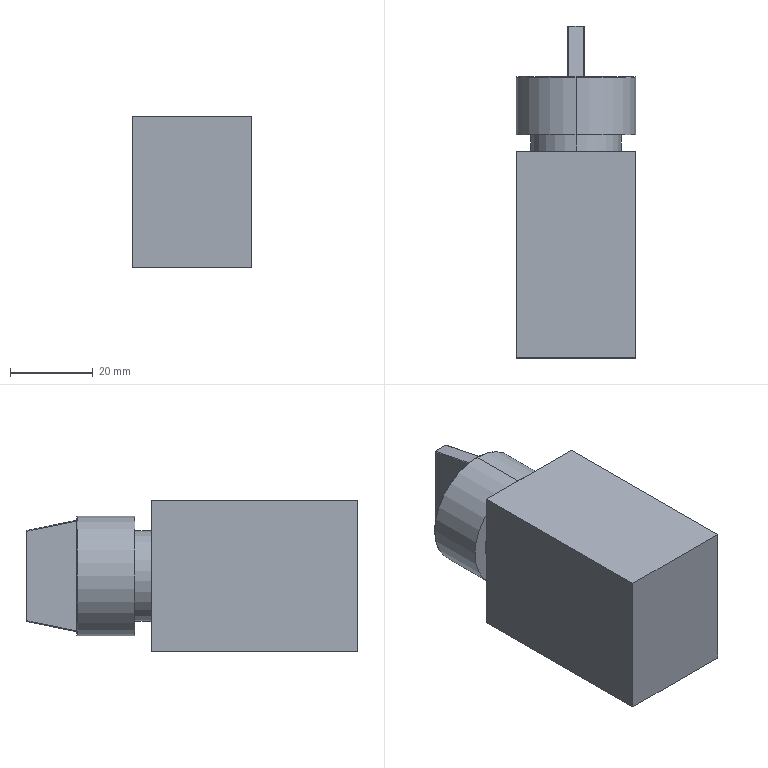Part | SolidWorks | features ICE 4, Extrusion 1, Fillet 1 | 1 solid | 25 faces | box 29 x 80.3 x 36.6 mm | volume 65042 mm3 | plane 13 | cylinder 10 | torus 2 | commonest cylinder face diameters 0.4 x6 22 x2 29 x2
STEP:
#1=CARTESIAN_POINT('',(0.,13.8,-14.5));
#2=VERTEX_POINT('',#1);
#3=CARTESIAN_POINT('',(0.,13.8,14.5));
#4=VERTEX_POINT('',#3);
#5=CARTESIAN_POINT('',(0.,13.8,0.));
#6=DIRECTION('',(0.,-1.,0.));
#7=DIRECTION('',(0.,0.,1.));
#8=AXIS2_PLACEMENT_3D('',#5,#6,#7);
#9=CIRCLE('',#8,14.5);
#10=EDGE_CURVE('',#2,#4,#9,.T.);
#11=ORIENTED_EDGE('',*,*,#10,.F.);
#12=CARTESIAN_POINT('',(0.,14.,-14.3));
#13=VERTEX_POINT('',#12);
#14=CARTESIAN_POINT('',(0.,13.8,-14.3));
#15=DIRECTION('',(1.,0.,0.));
#16=DIRECTION('',(0.,0.,-1.));
#17=AXIS2_PLACEMENT_3D('',#14,#15,#16);
#18=CIRCLE('',#17,0.2);
#19=EDGE_CURVE('',#2,#13,#18,.T.);
#20=ORIENTED_EDGE('',*,*,#19,.T.);
#21=CARTESIAN_POINT('',(0.,14.,14.3));
#22=VERTEX_POINT('',#21);
#23=CARTESIAN_POINT('',(0.,14.,0.));
#24=DIRECTION('',(0.,1.,0.));
#25=DIRECTION('',(0.,0.,1.));
#26=AXIS2_PLACEMENT_3D('',#23,#24,#25);
#27=CIRCLE('',#26,14.3);
#28=EDGE_CURVE('',#22,#13,#27,.T.);
#29=ORIENTED_EDGE('',*,*,#28,.F.);
#30=CARTESIAN_POINT('',(0.,13.8,14.3));
#31=DIRECTION('',(-1.,0.,0.));
#32=DIRECTION('',(0.,0.,1.));
#33=AXIS2_PLACEMENT_3D('',#30,#31,#32);
#34=CIRCLE('',#33,0.2);
#35=EDGE_CURVE('',#4,#22,#34,.T.);
#36=ORIENTED_EDGE('',*,*,#35,.F.);
#37=EDGE_LOOP('',(#11,#20,#29,#36));
#38=FACE_OUTER_BOUND('',#37,.T.);
#39=CARTESIAN_POINT('',(0.,13.8,0.));
#40=DIRECTION('',(0.,1.,0.));
#41=DIRECTION('',(0.,0.,1.));
#42=AXIS2_PLACEMENT_3D('',#39,#40,#41);
#43=TOROIDAL_SURFACE('',#42,14.3,0.2);
#44=ADVANCED_FACE('',(#38),#43,.T.);
#45=CARTESIAN_POINT('',(0.,-4.,-11.));
#46=VERTEX_POINT('',#45);
#47=CARTESIAN_POINT('',(0.,-4.,11.));
#48=VERTEX_POINT('',#47);
#49=CARTESIAN_POINT('',(0.,-4.,0.));
#50=DIRECTION('',(0.,-1.,0.));
#51=DIRECTION('',(0.,0.,-1.));
#52=AXIS2_PLACEMENT_3D('',#49,#50,#51);
#53=CIRCLE('',#52,11.);
#54=EDGE_CURVE('',#46,#48,#53,.T.);
#55=ORIENTED_EDGE('',*,*,#54,.F.);
#56=CARTESIAN_POINT('',(0.,0.,-11.));
#57=VERTEX_POINT('',#56);
#58=CARTESIAN_POINT('',(0.,-4.,-11.));
#59=DIRECTION('',(0.,1.,0.));
#60=VECTOR('',#59,1000.);
#61=LINE('',#58,#60);
#62=EDGE_CURVE('',#46,#57,#61,.T.);
#63=ORIENTED_EDGE('',*,*,#62,.T.);
#64=CARTESIAN_POINT('',(0.,0.,11.));
#65=VERTEX_POINT('',#64);
#66=CARTESIAN_POINT('',(0.,0.,0.));
#67=DIRECTION('',(0.,-1.,0.));
#68=DIRECTION('',(0.,0.,1.));
#69=AXIS2_PLACEMENT_3D('',#66,#67,#68);
#70=CIRCLE('',#69,11.);
#71=EDGE_CURVE('',#57,#65,#70,.T.);
#72=ORIENTED_EDGE('',*,*,#71,.T.);
#73=CARTESIAN_POINT('',(0.,-4.,11.));
#74=DIRECTION('',(0.,1.,0.));
#75=VECTOR('',#74,1000.);
#76=LINE('',#73,#75);
#77=EDGE_CURVE('',#48,#65,#76,.T.);
#78=ORIENTED_EDGE('',*,*,#77,.F.);
#79=EDGE_LOOP('',(#55,#63,#72,#78));
#80=FACE_OUTER_BOUND('',#79,.T.);
#81=CARTESIAN_POINT('',(0.,-4.,0.));
#82=DIRECTION('',(0.,1.,0.));
#83=DIRECTION('',(0.,0.,1.));
#84=AXIS2_PLACEMENT_3D('',#81,#82,#83);
#85=CYLINDRICAL_SURFACE('',#84,11.);
#86=ADVANCED_FACE('',(#80),#85,.T.);
#87=ORIENTED_EDGE('',*,*,#10,.T.);
#88=CARTESIAN_POINT('',(0.,0.,14.5));
#89=VERTEX_POINT('',#88);
#90=CARTESIAN_POINT('',(0.,14.,14.5));
#91=DIRECTION('',(0.,-1.,0.));
#92=VECTOR('',#91,1000.);
#93=LINE('',#90,#92);
#94=EDGE_CURVE('',#4,#89,#93,.T.);
#95=ORIENTED_EDGE('',*,*,#94,.T.);
#96=CARTESIAN_POINT('',(0.,0.,-14.5));
#97=VERTEX_POINT('',#96);
#98=CARTESIAN_POINT('',(0.,0.,0.));
#99=DIRECTION('',(0.,1.,0.));
#100=DIRECTION('',(0.,0.,1.));
#101=AXIS2_PLACEMENT_3D('',#98,#99,#100);
#102=CIRCLE('',#101,14.5);
#103=EDGE_CURVE('',#89,#97,#102,.T.);
#104=ORIENTED_EDGE('',*,*,#103,.T.);
#105=CARTESIAN_POINT('',(0.,14.,-14.5));
#106=DIRECTION('',(0.,-1.,0.));
#107=VECTOR('',#106,1000.);
#108=LINE('',#105,#107);
#109=EDGE_CURVE('',#2,#97,#108,.T.);
#110=ORIENTED_EDGE('',*,*,#109,.F.);
#111=EDGE_LOOP('',(#87,#95,#104,#110));
#112=FACE_OUTER_BOUND('',#111,.T.);
#113=CARTESIAN_POINT('',(0.,14.,0.));
#114=DIRECTION('',(0.,-1.,0.));
#115=DIRECTION('',(0.,0.,-1.));
#116=AXIS2_PLACEMENT_3D('',#113,#114,#115);
#117=CYLINDRICAL_SURFACE('',#116,14.5);
#118=ADVANCED_FACE('',(#112),#117,.T.);
#119=CARTESIAN_POINT('',(0.,0.,0.));
#120=DIRECTION('',(0.,1.,0.));
#121=DIRECTION('',(0.,0.,1.));
#122=AXIS2_PLACEMENT_3D('',#119,#120,#121);
#123=CIRCLE('',#122,14.5);
#124=EDGE_CURVE('',#97,#89,#123,.T.);
#125=ORIENTED_EDGE('',*,*,#124,.F.);
#126=ORIENTED_EDGE('',*,*,#103,.F.);
#127=EDGE_LOOP('',(#125,#126));
#128=FACE_OUTER_BOUND('',#127,.T.);
#129=CARTESIAN_POINT('',(0.,0.,0.));
#130=DIRECTION('',(0.,-1.,0.));
#131=DIRECTION('',(0.,0.,1.));
#132=AXIS2_PLACEMENT_3D('',#129,#130,#131);
#133=CIRCLE('',#132,11.);
#134=EDGE_CURVE('',#65,#57,#133,.T.);
#135=ORIENTED_EDGE('',*,*,#134,.F.);
#136=ORIENTED_EDGE('',*,*,#71,.F.);
#137=EDGE_LOOP('',(#135,#136));
#138=FACE_BOUND('',#137,.T.);
#139=CARTESIAN_POINT('',(0.,0.,0.));
#140=DIRECTION('',(0.,1.,0.));
#141=DIRECTION('',(0.,0.,1.));
#142=AXIS2_PLACEMENT_3D('',#139,#140,#141);
#143=PLANE('',#142);
#144=ADVANCED_FACE('',(#128,#138),#143,.F.);
#145=ORIENTED_EDGE('',*,*,#28,.T.);
#146=CARTESIAN_POINT('',(0.,14.,0.));
#147=DIRECTION('',(0.,1.,0.));
#148=DIRECTION('',(0.,0.,1.));
#149=AXIS2_PLACEMENT_3D('',#146,#147,#148);
#150=CIRCLE('',#149,14.3);
#151=EDGE_CURVE('',#13,#22,#150,.T.);
#152=ORIENTED_EDGE('',*,*,#151,.T.);
#153=EDGE_LOOP('',(#145,#152));
#154=FACE_OUTER_BOUND('',#153,.T.);
#155=CARTESIAN_POINT('',(-1.8,14.,13.5));
#156=VERTEX_POINT('',#155);
#157=CARTESIAN_POINT('',(1.8,14.,13.5));
#158=VERTEX_POINT('',#157);
#159=CARTESIAN_POINT('',(-2.,14.,13.5));
#160=DIRECTION('',(1.,0.,0.));
#161=VECTOR('',#160,1000.);
#162=LINE('',#159,#161);
#163=EDGE_CURVE('',#156,#158,#162,.T.);
#164=ORIENTED_EDGE('',*,*,#163,.F.);
#165=CARTESIAN_POINT('',(-2.,14.,13.296));
#166=VERTEX_POINT('',#165);
#167=CARTESIAN_POINT('',(-1.8,14.,13.5));
#168=CARTESIAN_POINT('',(-1.917,14.,13.5));
#169=CARTESIAN_POINT('',(-2.,14.,13.415));
#170=CARTESIAN_POINT('',(-2.,14.,13.296));
#171=(BOUNDED_CURVE()B_SPLINE_CURVE(3,(#167,#168,#169,#170),.UNSPECIFIED.,.F.,.F.)B_SPLINE_CURVE_WITH_KNOTS((4,4),(3.142,4.712),.UNSPECIFIED.)CURVE()GEOMETRIC_REPRESENTATION_ITEM()RATIONAL_B_SPLINE_CURVE((1.,0.8047,0.8047,1.))REPRESENTATION_ITEM(''));
#172=EDGE_CURVE('',#156,#166,#171,.T.);
#173=ORIENTED_EDGE('',*,*,#172,.T.);
#174=CARTESIAN_POINT('',(-2.,14.,-13.296));
#175=VERTEX_POINT('',#174);
#176=CARTESIAN_POINT('',(-2.,14.,13.5));
#177=DIRECTION('',(0.,0.,1.));
#178=VECTOR('',#177,1000.);
#179=LINE('',#176,#178);
#180=EDGE_CURVE('',#175,#166,#179,.T.);
#181=ORIENTED_EDGE('',*,*,#180,.F.);
#182=CARTESIAN_POINT('',(-1.8,14.,-13.5));
#183=VERTEX_POINT('',#182);
#184=CARTESIAN_POINT('',(-2.,14.,-13.296));
#185=CARTESIAN_POINT('',(-2.,14.,-13.415));
#186=CARTESIAN_POINT('',(-1.917,14.,-13.5));
#187=CARTESIAN_POINT('',(-1.8,14.,-13.5));
#188=(BOUNDED_CURVE()B_SPLINE_CURVE(3,(#184,#185,#186,#187),.UNSPECIFIED.,.F.,.T.)B_SPLINE_CURVE_WITH_KNOTS((4,4),(4.712,6.283),.UNSPECIFIED.)CURVE()GEOMETRIC_REPRESENTATION_ITEM()RATIONAL_B_SPLINE_CURVE((1.,0.8047,0.8047,1.))REPRESENTATION_ITEM(''));
#189=EDGE_CURVE('',#175,#183,#188,.T.);
#190=ORIENTED_EDGE('',*,*,#189,.T.);
#191=CARTESIAN_POINT('',(1.8,14.,-13.5));
#192=VERTEX_POINT('',#191);
#193=CARTESIAN_POINT('',(-2.,14.,-13.5));
#194=DIRECTION('',(-1.,0.,0.));
#195=VECTOR('',#194,1000.);
#196=LINE('',#193,#195);
#197=EDGE_CURVE('',#192,#183,#196,.T.);
#198=ORIENTED_EDGE('',*,*,#197,.F.);
#199=CARTESIAN_POINT('',(2.,14.,-13.296));
#200=VERTEX_POINT('',#199);
#201=CARTESIAN_POINT('',(1.8,14.,-13.5));
#202=CARTESIAN_POINT('',(1.917,14.,-13.5));
#203=CARTESIAN_POINT('',(2.,14.,-13.415));
#204=CARTESIAN_POINT('',(2.,14.,-13.296));
#205=(BOUNDED_CURVE()B_SPLINE_CURVE(3,(#201,#202,#203,#204),.UNSPECIFIED.,.F.,.F.)B_SPLINE_CURVE_WITH_KNOTS((4,4),(0.,1.571),.UNSPECIFIED.)CURVE()GEOMETRIC_REPRESENTATION_ITEM()RATIONAL_B_SPLINE_CURVE((1.,0.8047,0.8047,1.))REPRESENTATION_ITEM(''));
#206=EDGE_CURVE('',#192,#200,#205,.T.);
#207=ORIENTED_EDGE('',*,*,#206,.T.);
#208=CARTESIAN_POINT('',(2.,14.,13.296));
#209=VERTEX_POINT('',#208);
#210=CARTESIAN_POINT('',(2.,14.,13.5));
#211=DIRECTION('',(0.,0.,-1.));
#212=VECTOR('',#211,1000.);
#213=LINE('',#210,#212);
#214=EDGE_CURVE('',#209,#200,#213,.T.);
#215=ORIENTED_EDGE('',*,*,#214,.F.);
#216=CARTESIAN_POINT('',(2.,14.,13.296));
#217=CARTESIAN_POINT('',(2.,14.,13.415));
#218=CARTESIAN_POINT('',(1.917,14.,13.5));
#219=CARTESIAN_POINT('',(1.8,14.,13.5));
#220=(BOUNDED_CURVE()B_SPLINE_CURVE(3,(#216,#217,#218,#219),.UNSPECIFIED.,.F.,.T.)B_SPLINE_CURVE_WITH_KNOTS((4,4),(1.571,3.142),.UNSPECIFIED.)CURVE()GEOMETRIC_REPRESENTATION_ITEM()RATIONAL_B_SPLINE_CURVE((1.,0.8047,0.8047,1.))REPRESENTATION_ITEM(''));
#221=EDGE_CURVE('',#209,#158,#220,.T.);
#222=ORIENTED_EDGE('',*,*,#221,.T.);
#223=EDGE_LOOP('',(#164,#173,#181,#190,#198,#207,#215,#222));
#224=FACE_BOUND('',#223,.T.);
#225=CARTESIAN_POINT('',(0.,14.,0.));
#226=DIRECTION('',(0.,1.,0.));
#227=DIRECTION('',(0.,0.,1.));
#228=AXIS2_PLACEMENT_3D('',#225,#226,#227);
#229=PLANE('',#228);
#230=ADVANCED_FACE('',(#154,#224),#229,.T.);
#231=ORIENTED_EDGE('',*,*,#94,.F.);
#232=CARTESIAN_POINT('',(0.,13.8,0.));
#233=DIRECTION('',(0.,-1.,0.));
#234=DIRECTION('',(0.,0.,1.));
#235=AXIS2_PLACEMENT_3D('',#232,#233,#234);
#236=CIRCLE('',#235,14.5);
#237=EDGE_CURVE('',#4,#2,#236,.T.);
#238=ORIENTED_EDGE('',*,*,#237,.T.);
#239=ORIENTED_EDGE('',*,*,#109,.T.);
#240=ORIENTED_EDGE('',*,*,#124,.T.);
#241=EDGE_LOOP('',(#231,#238,#239,#240));
#242=FACE_OUTER_BOUND('',#241,.T.);
#243=CARTESIAN_POINT('',(0.,14.,0.));
#244=DIRECTION('',(0.,-1.,0.));
#245=DIRECTION('',(0.,0.,-1.));
#246=AXIS2_PLACEMENT_3D('',#243,#244,#245);
#247=CYLINDRICAL_SURFACE('',#246,14.5);
#248=ADVANCED_FACE('',(#242),#247,.T.);
#249=CARTESIAN_POINT('',(2.,26.1,-10.837));
#250=VERTEX_POINT('',#249);
#251=CARTESIAN_POINT('',(2.,26.1,10.837));
#252=VERTEX_POINT('',#251);
#253=CARTESIAN_POINT('',(2.,26.1,13.5));
#254=DIRECTION('',(0.,0.,1.));
#255=VECTOR('',#254,1000.);
#256=LINE('',#253,#255);
#257=EDGE_CURVE('',#250,#252,#256,.T.);
#258=ORIENTED_EDGE('',*,*,#257,.T.);
#259=CARTESIAN_POINT('',(2.,25.772,10.903));
#260=DIRECTION('',(0.,-0.98,0.1992));
#261=VECTOR('',#260,1000.);
#262=LINE('',#259,#261);
#263=EDGE_CURVE('',#252,#209,#262,.T.);
#264=ORIENTED_EDGE('',*,*,#263,.T.);
#265=ORIENTED_EDGE('',*,*,#214,.T.);
#266=CARTESIAN_POINT('',(2.,31.042,-9.832));
#267=DIRECTION('',(0.,0.98,0.1992));
#268=VECTOR('',#267,1000.);
#269=LINE('',#266,#268);
#270=EDGE_CURVE('',#200,#250,#269,.T.);
#271=ORIENTED_EDGE('',*,*,#270,.T.);
#272=EDGE_LOOP('',(#258,#264,#265,#271));
#273=FACE_OUTER_BOUND('',#272,.T.);
#274=CARTESIAN_POINT('',(2.,26.3,13.5));
#275=DIRECTION('',(-1.,0.,0.));
#276=DIRECTION('',(0.,0.,1.));
#277=AXIS2_PLACEMENT_3D('',#274,#275,#276);
#278=PLANE('',#277);
#279=ADVANCED_FACE('',(#273),#278,.F.);
#280=ORIENTED_EDGE('',*,*,#180,.T.);
#281=CARTESIAN_POINT('',(-2.,26.1,10.837));
#282=VERTEX_POINT('',#281);
#283=CARTESIAN_POINT('',(-2.,25.772,10.903));
#284=DIRECTION('',(0.,0.98,-0.1992));
#285=VECTOR('',#284,1000.);
#286=LINE('',#283,#285);
#287=EDGE_CURVE('',#166,#282,#286,.T.);
#288=ORIENTED_EDGE('',*,*,#287,.T.);
#289=CARTESIAN_POINT('',(-2.,26.1,-10.837));
#290=VERTEX_POINT('',#289);
#291=CARTESIAN_POINT('',(-2.,26.1,13.5));
#292=DIRECTION('',(0.,0.,-1.));
#293=VECTOR('',#292,1000.);
#294=LINE('',#291,#293);
#295=EDGE_CURVE('',#282,#290,#294,.T.);
#296=ORIENTED_EDGE('',*,*,#295,.T.);
#297=CARTESIAN_POINT('',(-2.,31.042,-9.832));
#298=DIRECTION('',(0.,-0.98,-0.1992));
#299=VECTOR('',#298,1000.);
#300=LINE('',#297,#299);
#301=EDGE_CURVE('',#290,#175,#300,.T.);
#302=ORIENTED_EDGE('',*,*,#301,.T.);
#303=EDGE_LOOP('',(#280,#288,#296,#302));
#304=FACE_OUTER_BOUND('',#303,.T.);
#305=CARTESIAN_POINT('',(-2.,26.3,13.5));
#306=DIRECTION('',(1.,0.,0.));
#307=DIRECTION('',(0.,0.,-1.));
#308=AXIS2_PLACEMENT_3D('',#305,#306,#307);
#309=PLANE('',#308);
#310=ADVANCED_FACE('',(#304),#309,.F.);
#311=CARTESIAN_POINT('',(-1.8,26.3,11.));
#312=VERTEX_POINT('',#311);
#313=CARTESIAN_POINT('',(1.8,26.3,11.));
#314=VERTEX_POINT('',#313);
#315=CARTESIAN_POINT('',(2.,26.3,11.));
#316=DIRECTION('',(1.,0.,0.));
#317=VECTOR('',#316,1000.);
#318=LINE('',#315,#317);
#319=EDGE_CURVE('',#312,#314,#318,.T.);
#320=ORIENTED_EDGE('',*,*,#319,.T.);
#321=CARTESIAN_POINT('',(1.8,26.3,-11.));
#322=VERTEX_POINT('',#321);
#323=CARTESIAN_POINT('',(1.8,26.3,-13.5));
#324=DIRECTION('',(0.,0.,-1.));
#325=VECTOR('',#324,1000.);
#326=LINE('',#323,#325);
#327=EDGE_CURVE('',#314,#322,#326,.T.);
#328=ORIENTED_EDGE('',*,*,#327,.T.);
#329=CARTESIAN_POINT('',(-1.8,26.3,-11.));
#330=VERTEX_POINT('',#329);
#331=CARTESIAN_POINT('',(2.,26.3,-11.));
#332=DIRECTION('',(-1.,0.,0.));
#333=VECTOR('',#332,1000.);
#334=LINE('',#331,#333);
#335=EDGE_CURVE('',#322,#330,#334,.T.);
#336=ORIENTED_EDGE('',*,*,#335,.T.);
#337=CARTESIAN_POINT('',(-1.8,26.3,-13.5));
#338=DIRECTION('',(0.,0.,1.));
#339=VECTOR('',#338,1000.);
#340=LINE('',#337,#339);
#341=EDGE_CURVE('',#330,#312,#340,.T.);
#342=ORIENTED_EDGE('',*,*,#341,.T.);
#343=EDGE_LOOP('',(#320,#328,#336,#342));
#344=FACE_OUTER_BOUND('',#343,.T.);
#345=CARTESIAN_POINT('',(2.,26.3,-13.5));
#346=DIRECTION('',(0.,-1.,0.));
#347=DIRECTION('',(0.,0.,-1.));
#348=AXIS2_PLACEMENT_3D('',#345,#346,#347);
#349=PLANE('',#348);
#350=ADVANCED_FACE('',(#344),#349,.F.);
#351=ORIENTED_EDGE('',*,*,#163,.T.);
#352=CARTESIAN_POINT('',(1.8,14.,13.5));
#353=DIRECTION('',(0.,0.98,-0.1992));
#354=VECTOR('',#353,1000.);
#355=LINE('',#352,#354);
#356=EDGE_CURVE('',#158,#314,#355,.T.);
#357=ORIENTED_EDGE('',*,*,#356,.T.);
#358=ORIENTED_EDGE('',*,*,#319,.F.);
#359=CARTESIAN_POINT('',(-1.8,14.,13.5));
#360=DIRECTION('',(0.,-0.98,0.1992));
#361=VECTOR('',#360,1000.);
#362=LINE('',#359,#361);
#363=EDGE_CURVE('',#312,#156,#362,.T.);
#364=ORIENTED_EDGE('',*,*,#363,.T.);
#365=EDGE_LOOP('',(#351,#357,#358,#364));
#366=FACE_OUTER_BOUND('',#365,.T.);
#367=CARTESIAN_POINT('',(-10.3,14.,13.5));
#368=DIRECTION('',(0.,-0.1992,-0.98));
#369=DIRECTION('',(0.,0.98,-0.1992));
#370=AXIS2_PLACEMENT_3D('',#367,#368,#369);
#371=PLANE('',#370);
#372=ADVANCED_FACE('',(#366),#371,.F.);
#373=ORIENTED_EDGE('',*,*,#335,.F.);
#374=CARTESIAN_POINT('',(1.8,14.,-13.5));
#375=DIRECTION('',(0.,-0.98,-0.1992));
#376=VECTOR('',#375,1000.);
#377=LINE('',#374,#376);
#378=EDGE_CURVE('',#322,#192,#377,.T.);
#379=ORIENTED_EDGE('',*,*,#378,.T.);
#380=ORIENTED_EDGE('',*,*,#197,.T.);
#381=CARTESIAN_POINT('',(-1.8,14.,-13.5));
#382=DIRECTION('',(0.,0.98,0.1992));
#383=VECTOR('',#382,1000.);
#384=LINE('',#381,#383);
#385=EDGE_CURVE('',#183,#330,#384,.T.);
#386=ORIENTED_EDGE('',*,*,#385,.T.);
#387=EDGE_LOOP('',(#373,#379,#380,#386));
#388=FACE_OUTER_BOUND('',#387,.T.);
#389=CARTESIAN_POINT('',(-10.3,14.,-13.5));
#390=DIRECTION('',(0.,-0.1992,0.98));
#391=DIRECTION('',(0.,-0.98,-0.1992));
#392=AXIS2_PLACEMENT_3D('',#389,#390,#391);
#393=PLANE('',#392);
#394=ADVANCED_FACE('',(#388),#393,.F.);
#395=ORIENTED_EDGE('',*,*,#62,.F.);
#396=CARTESIAN_POINT('',(0.,-4.,0.));
#397=DIRECTION('',(0.,-1.,0.));
#398=DIRECTION('',(0.,0.,-1.));
#399=AXIS2_PLACEMENT_3D('',#396,#397,#398);
#400=CIRCLE('',#399,11.);
#401=EDGE_CURVE('',#48,#46,#400,.T.);
#402=ORIENTED_EDGE('',*,*,#401,.F.);
#403=ORIENTED_EDGE('',*,*,#77,.T.);
#404=ORIENTED_EDGE('',*,*,#134,.T.);
#405=EDGE_LOOP('',(#395,#402,#403,#404));
#406=FACE_OUTER_BOUND('',#405,.T.);
#407=CARTESIAN_POINT('',(0.,-4.,0.));
#408=DIRECTION('',(0.,1.,0.));
#409=DIRECTION('',(0.,0.,1.));
#410=AXIS2_PLACEMENT_3D('',#407,#408,#409);
#411=CYLINDRICAL_SURFACE('',#410,11.);
#412=ADVANCED_FACE('',(#406),#411,.T.);
#413=CARTESIAN_POINT('',(14.5,-4.,-18.3));
#414=VERTEX_POINT('',#413);
#415=CARTESIAN_POINT('',(14.5,-4.,18.3));
#416=VERTEX_POINT('',#415);
#417=CARTESIAN_POINT('',(14.5,-4.,-18.3));
#418=DIRECTION('',(0.,0.,1.));
#419=VECTOR('',#418,1000.);
#420=LINE('',#417,#419);
#421=EDGE_CURVE('',#414,#416,#420,.T.);
#422=ORIENTED_EDGE('',*,*,#421,.F.);
#423=CARTESIAN_POINT('',(-14.5,-4.,-18.3));
#424=VERTEX_POINT('',#423);
#425=CARTESIAN_POINT('',(-14.5,-4.,-18.3));
#426=DIRECTION('',(1.,0.,0.));
#427=VECTOR('',#426,1000.);
#428=LINE('',#425,#427);
#429=EDGE_CURVE('',#424,#414,#428,.T.);
#430=ORIENTED_EDGE('',*,*,#429,.F.);
#431=CARTESIAN_POINT('',(-14.5,-4.,18.3));
#432=VERTEX_POINT('',#431);
#433=CARTESIAN_POINT('',(-14.5,-4.,-18.3));
#434=DIRECTION('',(0.,0.,-1.));
#435=VECTOR('',#434,1000.);
#436=LINE('',#433,#435);
#437=EDGE_CURVE('',#432,#424,#436,.T.);
#438=ORIENTED_EDGE('',*,*,#437,.F.);
#439=CARTESIAN_POINT('',(-14.5,-4.,18.3));
#440=DIRECTION('',(-1.,0.,0.));
#441=VECTOR('',#440,1000.);
#442=LINE('',#439,#441);
#443=EDGE_CURVE('',#416,#432,#442,.T.);
#444=ORIENTED_EDGE('',*,*,#443,.F.);
#445=EDGE_LOOP('',(#422,#430,#438,#444));
#446=FACE_OUTER_BOUND('',#445,.T.);
#447=ORIENTED_EDGE('',*,*,#401,.T.);
#448=ORIENTED_EDGE('',*,*,#54,.T.);
#449=EDGE_LOOP('',(#447,#448));
#450=FACE_BOUND('',#449,.T.);
#451=CARTESIAN_POINT('',(14.5,-4.,18.3));
#452=DIRECTION('',(0.,1.,0.));
#453=DIRECTION('',(0.,0.,1.));
#454=AXIS2_PLACEMENT_3D('',#451,#452,#453);
#455=PLANE('',#454);
#456=ADVANCED_FACE('',(#446,#450),#455,.T.);
#457=ORIENTED_EDGE('',*,*,#421,.T.);
#458=CARTESIAN_POINT('',(14.5,-54.,18.3));
#459=VERTEX_POINT('',#458);
#460=CARTESIAN_POINT('',(14.5,-54.,18.3));
#461=DIRECTION('',(0.,1.,0.));
#462=VECTOR('',#461,1000.);
#463=LINE('',#460,#462);
#464=EDGE_CURVE('',#459,#416,#463,.T.);
#465=ORIENTED_EDGE('',*,*,#464,.F.);
#466=CARTESIAN_POINT('',(14.5,-54.,-18.3));
#467=VERTEX_POINT('',#466);
#468=CARTESIAN_POINT('',(14.5,-54.,-18.3));
#469=DIRECTION('',(0.,0.,1.));
#470=VECTOR('',#469,1000.);
#471=LINE('',#468,#470);
#472=EDGE_CURVE('',#467,#459,#471,.T.);
#473=ORIENTED_EDGE('',*,*,#472,.F.);
#474=CARTESIAN_POINT('',(14.5,-54.,-18.3));
#475=DIRECTION('',(0.,1.,0.));
#476=VECTOR('',#475,1000.);
#477=LINE('',#474,#476);
#478=EDGE_CURVE('',#467,#414,#477,.T.);
#479=ORIENTED_EDGE('',*,*,#478,.T.);
#480=EDGE_LOOP('',(#457,#465,#473,#479));
#481=FACE_OUTER_BOUND('',#480,.T.);
#482=CARTESIAN_POINT('',(14.5,-54.,-18.3));
#483=DIRECTION('',(-1.,0.,0.));
#484=DIRECTION('',(0.,0.,1.));
#485=AXIS2_PLACEMENT_3D('',#482,#483,#484);
#486=PLANE('',#485);
#487=ADVANCED_FACE('',(#481),#486,.F.);
#488=ORIENTED_EDGE('',*,*,#443,.T.);
#489=CARTESIAN_POINT('',(-14.5,-54.,18.3));
#490=VERTEX_POINT('',#489);
#491=CARTESIAN_POINT('',(-14.5,-54.,18.3));
#492=DIRECTION('',(0.,1.,0.));
#493=VECTOR('',#492,1000.);
#494=LINE('',#491,#493);
#495=EDGE_CURVE('',#490,#432,#494,.T.);
#496=ORIENTED_EDGE('',*,*,#495,.F.);
#497=CARTESIAN_POINT('',(-14.5,-54.,18.3));
#498=DIRECTION('',(-1.,0.,0.));
#499=VECTOR('',#498,1000.);
#500=LINE('',#497,#499);
#501=EDGE_CURVE('',#459,#490,#500,.T.);
#502=ORIENTED_EDGE('',*,*,#501,.F.);
#503=ORIENTED_EDGE('',*,*,#464,.T.);
#504=EDGE_LOOP('',(#488,#496,#502,#503));
#505=FACE_OUTER_BOUND('',#504,.T.);
#506=CARTESIAN_POINT('',(-14.5,-54.,18.3));
#507=DIRECTION('',(0.,0.,-1.));
#508=DIRECTION('',(-1.,0.,0.));
#509=AXIS2_PLACEMENT_3D('',#506,#507,#508);
#510=PLANE('',#509);
#511=ADVANCED_FACE('',(#505),#510,.F.);
#512=ORIENTED_EDGE('',*,*,#437,.T.);
#513=CARTESIAN_POINT('',(-14.5,-54.,-18.3));
#514=VERTEX_POINT('',#513);
#515=CARTESIAN_POINT('',(-14.5,-54.,-18.3));
#516=DIRECTION('',(0.,1.,0.));
#517=VECTOR('',#516,1000.);
#518=LINE('',#515,#517);
#519=EDGE_CURVE('',#514,#424,#518,.T.);
#520=ORIENTED_EDGE('',*,*,#519,.F.);
#521=CARTESIAN_POINT('',(-14.5,-54.,-18.3));
#522=DIRECTION('',(0.,0.,-1.));
#523=VECTOR('',#522,1000.);
#524=LINE('',#521,#523);
#525=EDGE_CURVE('',#490,#514,#524,.T.);
#526=ORIENTED_EDGE('',*,*,#525,.F.);
#527=ORIENTED_EDGE('',*,*,#495,.T.);
#528=EDGE_LOOP('',(#512,#520,#526,#527));
#529=FACE_OUTER_BOUND('',#528,.T.);
#530=CARTESIAN_POINT('',(-14.5,-54.,-18.3));
#531=DIRECTION('',(1.,0.,0.));
#532=DIRECTION('',(0.,0.,-1.));
#533=AXIS2_PLACEMENT_3D('',#530,#531,#532);
#534=PLANE('',#533);
#535=ADVANCED_FACE('',(#529),#534,.F.);
#536=ORIENTED_EDGE('',*,*,#429,.T.);
#537=ORIENTED_EDGE('',*,*,#478,.F.);
#538=CARTESIAN_POINT('',(-14.5,-54.,-18.3));
#539=DIRECTION('',(1.,0.,0.));
#540=VECTOR('',#539,1000.);
#541=LINE('',#538,#540);
#542=EDGE_CURVE('',#514,#467,#541,.T.);
#543=ORIENTED_EDGE('',*,*,#542,.F.);
#544=ORIENTED_EDGE('',*,*,#519,.T.);
#545=EDGE_LOOP('',(#536,#537,#543,#544));
#546=FACE_OUTER_BOUND('',#545,.T.);
#547=CARTESIAN_POINT('',(-14.5,-54.,-18.3));
#548=DIRECTION('',(0.,0.,1.));
#549=DIRECTION('',(1.,0.,0.));
#550=AXIS2_PLACEMENT_3D('',#547,#548,#549);
#551=PLANE('',#550);
#552=ADVANCED_FACE('',(#546),#551,.F.);
#553=ORIENTED_EDGE('',*,*,#472,.T.);
#554=ORIENTED_EDGE('',*,*,#501,.T.);
#555=ORIENTED_EDGE('',*,*,#525,.T.);
#556=ORIENTED_EDGE('',*,*,#542,.T.);
#557=EDGE_LOOP('',(#553,#554,#555,#556));
#558=FACE_OUTER_BOUND('',#557,.T.);
#559=CARTESIAN_POINT('',(14.5,-54.,18.3));
#560=DIRECTION('',(0.,1.,0.));
#561=DIRECTION('',(0.,0.,1.));
#562=AXIS2_PLACEMENT_3D('',#559,#560,#561);
#563=PLANE('',#562);
#564=ADVANCED_FACE('',(#558),#563,.F.);
#565=ORIENTED_EDGE('',*,*,#19,.F.);
#566=ORIENTED_EDGE('',*,*,#237,.F.);
#567=ORIENTED_EDGE('',*,*,#35,.T.);
#568=ORIENTED_EDGE('',*,*,#151,.F.);
#569=EDGE_LOOP('',(#565,#566,#567,#568));
#570=FACE_OUTER_BOUND('',#569,.T.);
#571=CARTESIAN_POINT('',(0.,13.8,0.));
#572=DIRECTION('',(0.,1.,0.));
#573=DIRECTION('',(0.,0.,1.));
#574=AXIS2_PLACEMENT_3D('',#571,#572,#573);
#575=TOROIDAL_SURFACE('',#574,14.3,0.2);
#576=ADVANCED_FACE('',(#570),#575,.T.);
#577=ORIENTED_EDGE('',*,*,#206,.F.);
#578=ORIENTED_EDGE('',*,*,#378,.F.);
#579=CARTESIAN_POINT('',(2.,26.1,-10.837));
#580=CARTESIAN_POINT('',(2.,26.217,-10.932));
#581=CARTESIAN_POINT('',(1.917,26.3,-11.));
#582=CARTESIAN_POINT('',(1.8,26.3,-11.));
#583=(BOUNDED_CURVE()B_SPLINE_CURVE(3,(#579,#580,#581,#582),.UNSPECIFIED.,.F.,.T.)B_SPLINE_CURVE_WITH_KNOTS((4,4),(1.571,3.142),.UNSPECIFIED.)CURVE()GEOMETRIC_REPRESENTATION_ITEM()RATIONAL_B_SPLINE_CURVE((1.,0.8047,0.8047,1.))REPRESENTATION_ITEM(''));
#584=EDGE_CURVE('',#250,#322,#583,.T.);
#585=ORIENTED_EDGE('',*,*,#584,.F.);
#586=ORIENTED_EDGE('',*,*,#270,.F.);
#587=EDGE_LOOP('',(#577,#578,#585,#586));
#588=FACE_OUTER_BOUND('',#587,.T.);
#589=CARTESIAN_POINT('',(1.8,13.96,-13.304));
#590=DIRECTION('',(0.,-0.98,-0.1992));
#591=DIRECTION('',(0.,0.1992,-0.98));
#592=AXIS2_PLACEMENT_3D('',#589,#590,#591);
#593=CYLINDRICAL_SURFACE('',#592,0.2);
#594=ADVANCED_FACE('',(#588),#593,.T.);
#595=ORIENTED_EDGE('',*,*,#584,.T.);
#596=ORIENTED_EDGE('',*,*,#327,.F.);
#597=CARTESIAN_POINT('',(2.,26.1,10.837));
#598=CARTESIAN_POINT('',(2.,26.217,10.932));
#599=CARTESIAN_POINT('',(1.917,26.3,11.));
#600=CARTESIAN_POINT('',(1.8,26.3,11.));
#601=(BOUNDED_CURVE()B_SPLINE_CURVE(3,(#597,#598,#599,#600),.UNSPECIFIED.,.F.,.F.)B_SPLINE_CURVE_WITH_KNOTS((4,4),(1.571,3.142),.UNSPECIFIED.)CURVE()GEOMETRIC_REPRESENTATION_ITEM()RATIONAL_B_SPLINE_CURVE((1.,0.8047,0.8047,1.))REPRESENTATION_ITEM(''));
#602=EDGE_CURVE('',#252,#314,#601,.T.);
#603=ORIENTED_EDGE('',*,*,#602,.F.);
#604=ORIENTED_EDGE('',*,*,#257,.F.);
#605=EDGE_LOOP('',(#595,#596,#603,#604));
#606=FACE_OUTER_BOUND('',#605,.T.);
#607=CARTESIAN_POINT('',(1.8,26.1,-13.5));
#608=DIRECTION('',(0.,0.,-1.));
#609=DIRECTION('',(-1.,0.,0.));
#610=AXIS2_PLACEMENT_3D('',#607,#608,#609);
#611=CYLINDRICAL_SURFACE('',#610,0.2);
#612=ADVANCED_FACE('',(#606),#611,.T.);
#613=ORIENTED_EDGE('',*,*,#221,.F.);
#614=ORIENTED_EDGE('',*,*,#263,.F.);
#615=ORIENTED_EDGE('',*,*,#602,.T.);
#616=ORIENTED_EDGE('',*,*,#356,.F.);
#617=EDGE_LOOP('',(#613,#614,#615,#616));
#618=FACE_OUTER_BOUND('',#617,.T.);
#619=CARTESIAN_POINT('',(1.8,13.96,13.304));
#620=DIRECTION('',(0.,0.98,-0.1992));
#621=DIRECTION('',(0.,0.1992,0.98));
#622=AXIS2_PLACEMENT_3D('',#619,#620,#621);
#623=CYLINDRICAL_SURFACE('',#622,0.2);
#624=ADVANCED_FACE('',(#618),#623,.T.);
#625=ORIENTED_EDGE('',*,*,#189,.F.);
#626=ORIENTED_EDGE('',*,*,#301,.F.);
#627=CARTESIAN_POINT('',(-1.8,26.3,-11.));
#628=CARTESIAN_POINT('',(-1.917,26.3,-11.));
#629=CARTESIAN_POINT('',(-2.,26.217,-10.932));
#630=CARTESIAN_POINT('',(-2.,26.1,-10.837));
#631=(BOUNDED_CURVE()B_SPLINE_CURVE(3,(#627,#628,#629,#630),.UNSPECIFIED.,.F.,.F.)B_SPLINE_CURVE_WITH_KNOTS((4,4),(3.142,4.712),.UNSPECIFIED.)CURVE()GEOMETRIC_REPRESENTATION_ITEM()RATIONAL_B_SPLINE_CURVE((1.,0.8047,0.8047,1.))REPRESENTATION_ITEM(''));
#632=EDGE_CURVE('',#330,#290,#631,.T.);
#633=ORIENTED_EDGE('',*,*,#632,.F.);
#634=ORIENTED_EDGE('',*,*,#385,.F.);
#635=EDGE_LOOP('',(#625,#626,#633,#634));
#636=FACE_OUTER_BOUND('',#635,.T.);
#637=CARTESIAN_POINT('',(-1.8,31.042,-9.832));
#638=DIRECTION('',(0.,-0.98,-0.1992));
#639=DIRECTION('',(0.,0.1992,-0.98));
#640=AXIS2_PLACEMENT_3D('',#637,#638,#639);
#641=CYLINDRICAL_SURFACE('',#640,0.2);
#642=ADVANCED_FACE('',(#636),#641,.T.);
#643=ORIENTED_EDGE('',*,*,#172,.F.);
#644=ORIENTED_EDGE('',*,*,#363,.F.);
#645=CARTESIAN_POINT('',(-2.,26.1,10.837));
#646=CARTESIAN_POINT('',(-2.,26.217,10.932));
#647=CARTESIAN_POINT('',(-1.917,26.3,11.));
#648=CARTESIAN_POINT('',(-1.8,26.3,11.));
#649=(BOUNDED_CURVE()B_SPLINE_CURVE(3,(#645,#646,#647,#648),.UNSPECIFIED.,.F.,.T.)B_SPLINE_CURVE_WITH_KNOTS((4,4),(4.712,6.283),.UNSPECIFIED.)CURVE()GEOMETRIC_REPRESENTATION_ITEM()RATIONAL_B_SPLINE_CURVE((1.,0.8047,0.8047,1.))REPRESENTATION_ITEM(''));
#650=EDGE_CURVE('',#282,#312,#649,.T.);
#651=ORIENTED_EDGE('',*,*,#650,.F.);
#652=ORIENTED_EDGE('',*,*,#287,.F.);
#653=EDGE_LOOP('',(#643,#644,#651,#652));
#654=FACE_OUTER_BOUND('',#653,.T.);
#655=CARTESIAN_POINT('',(-1.8,25.772,10.903));
#656=DIRECTION('',(0.,0.98,-0.1992));
#657=DIRECTION('',(0.,0.1992,0.98));
#658=AXIS2_PLACEMENT_3D('',#655,#656,#657);
#659=CYLINDRICAL_SURFACE('',#658,0.2);
#660=ADVANCED_FACE('',(#654),#659,.T.);
#661=ORIENTED_EDGE('',*,*,#632,.T.);
#662=ORIENTED_EDGE('',*,*,#295,.F.);
#663=ORIENTED_EDGE('',*,*,#650,.T.);
#664=ORIENTED_EDGE('',*,*,#341,.F.);
#665=EDGE_LOOP('',(#661,#662,#663,#664));
#666=FACE_OUTER_BOUND('',#665,.T.);
#667=CARTESIAN_POINT('',(-1.8,26.1,-13.5));
#668=DIRECTION('',(0.,0.,1.));
#669=DIRECTION('',(1.,0.,0.));
#670=AXIS2_PLACEMENT_3D('',#667,#668,#669);
#671=CYLINDRICAL_SURFACE('',#670,0.2);
#672=ADVANCED_FACE('',(#666),#671,.T.);
#673=CLOSED_SHELL('',(#44,#86,#118,#144,#230,#248,#279,#310,#350,#372,#394,#412,#456,#487,#511,#535,#552,#564,#576,#594,#612,#624,#642,#660,#672));
#674=MANIFOLD_SOLID_BREP('',#673);
#675=CARTESIAN_POINT('',(0.,0.,0.));
#676=DIRECTION('',(0.,0.,1.));
#677=DIRECTION('',(1.,0.,0.));
#678=AXIS2_PLACEMENT_3D('',#675,#676,#677);
#679=(LENGTH_UNIT()NAMED_UNIT(*)SI_UNIT(.MILLI.,.METRE.));
#680=UNCERTAINTY_MEASURE_WITH_UNIT(LENGTH_MEASURE(0.00001),#679,'','');
#681=(NAMED_UNIT(*)PLANE_ANGLE_UNIT()SI_UNIT($,.RADIAN.));
#682=(NAMED_UNIT(*)SI_UNIT($,.STERADIAN.)SOLID_ANGLE_UNIT());
#683=(GEOMETRIC_REPRESENTATION_CONTEXT(3)GLOBAL_UNCERTAINTY_ASSIGNED_CONTEXT((#680))GLOBAL_UNIT_ASSIGNED_CONTEXT((#679,#681,#682))REPRESENTATION_CONTEXT('',''));
#684=ADVANCED_BREP_SHAPE_REPRESENTATION('',(#674,#678),#683);